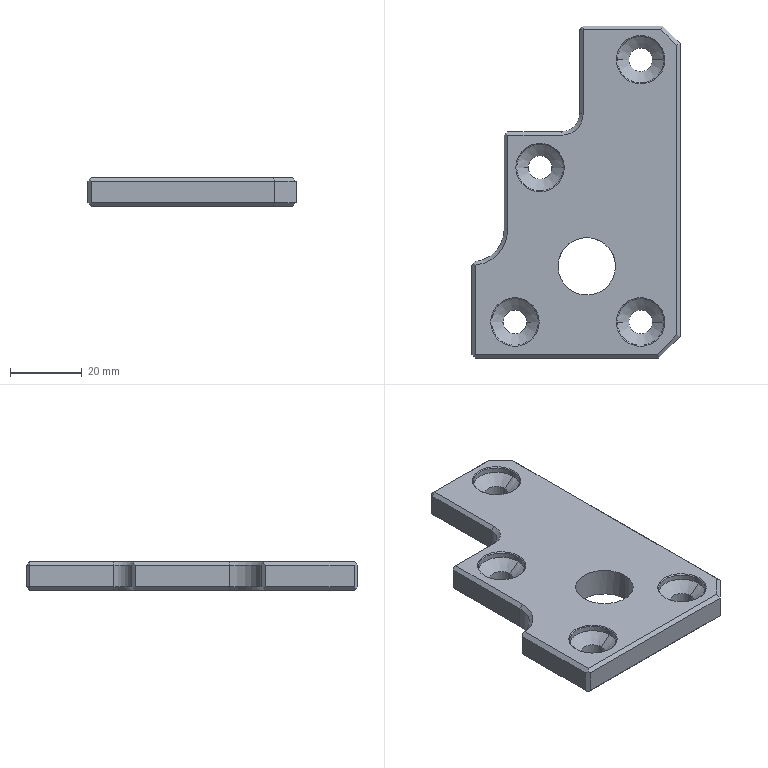Part | Creo | 1 solid | 77 faces | box 58 x 92.4 x 8 mm | volume 29001 mm3 | plane 37 | cone 20 | cylinder 20 | commonest cylinder face diameters 6.6 x8 13 x8 16 x2 10 x1 18 x1